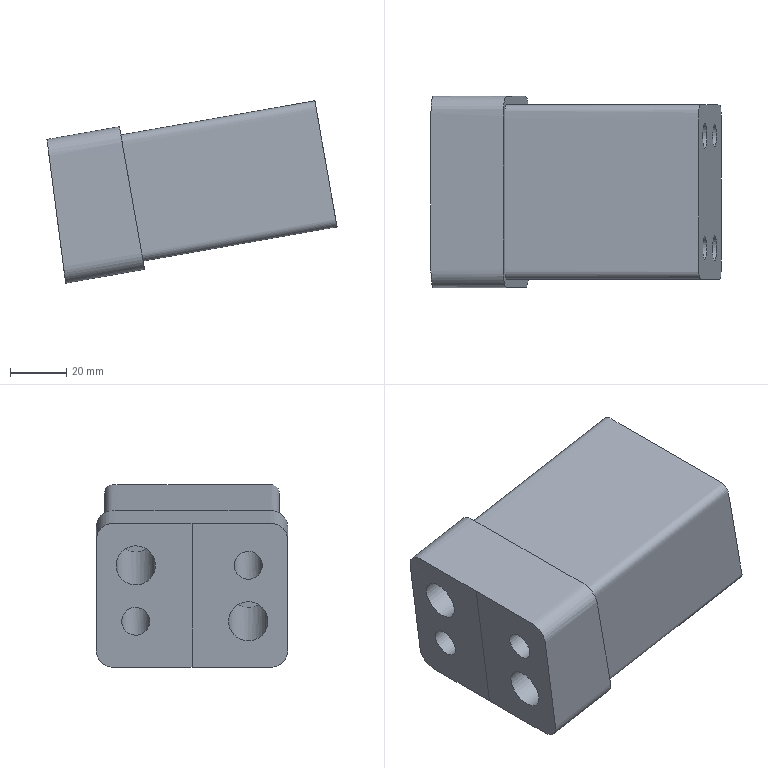Part | NX | features solid 2 | 1 solid | 18 faces | box 103.079 x 68.051 x 64.838 mm | volume 247029 mm3 | cylinder 8 | plane 6 | spline 4 | commonest cylinder face diameters 8 x2 9 x2 10 x2 14 x2